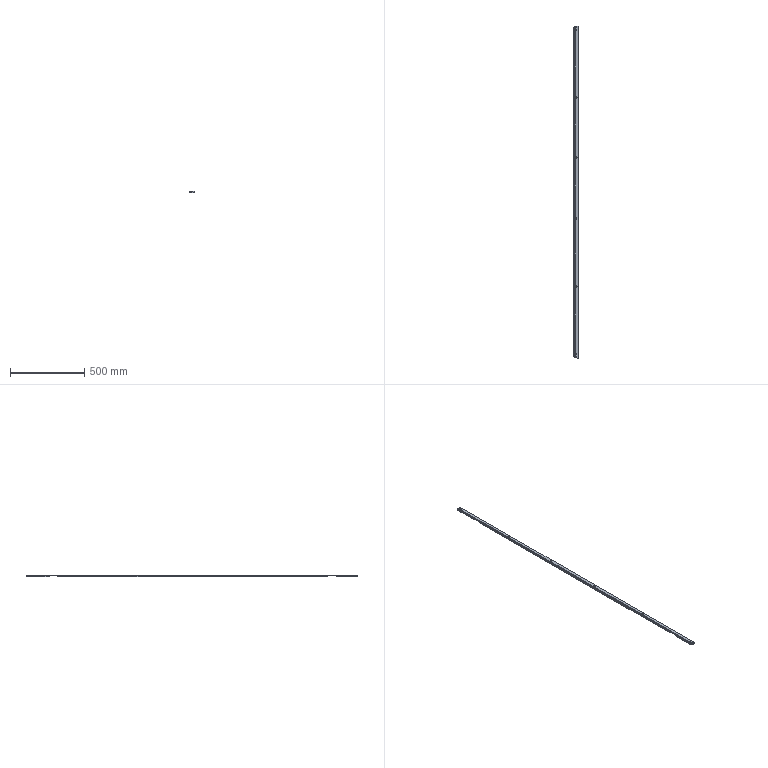Part | NX | features solid 2 | 1 solid | 79 faces | box 27.5 x 2236 x 10 mm | volume 555928 mm3 | plane 49 | cylinder 28 | cone 2 | commonest cylinder face diameters 8.2 x6 13.5 x6 4.5 x4 8 x4 20 x4 10.55 x2